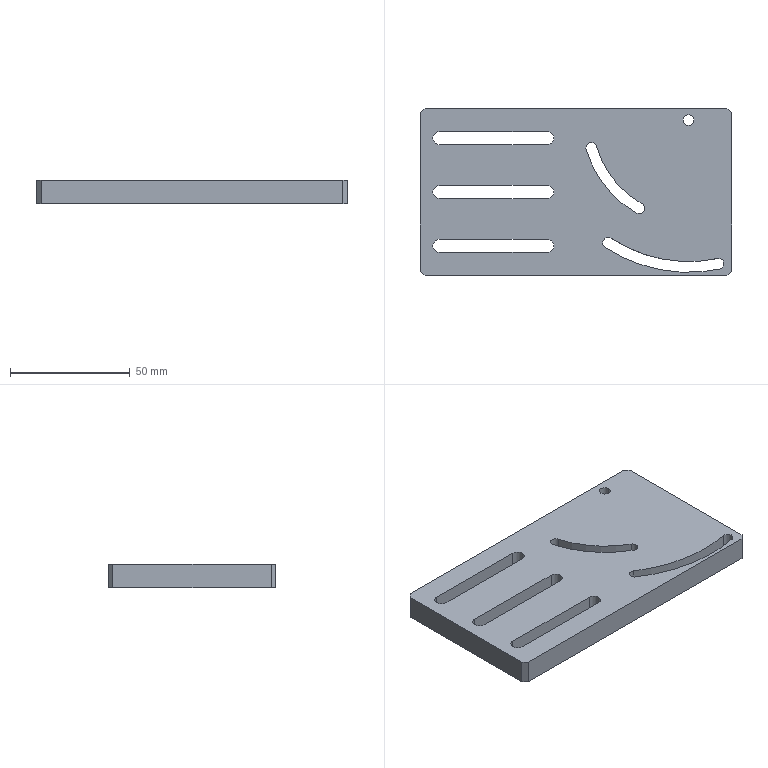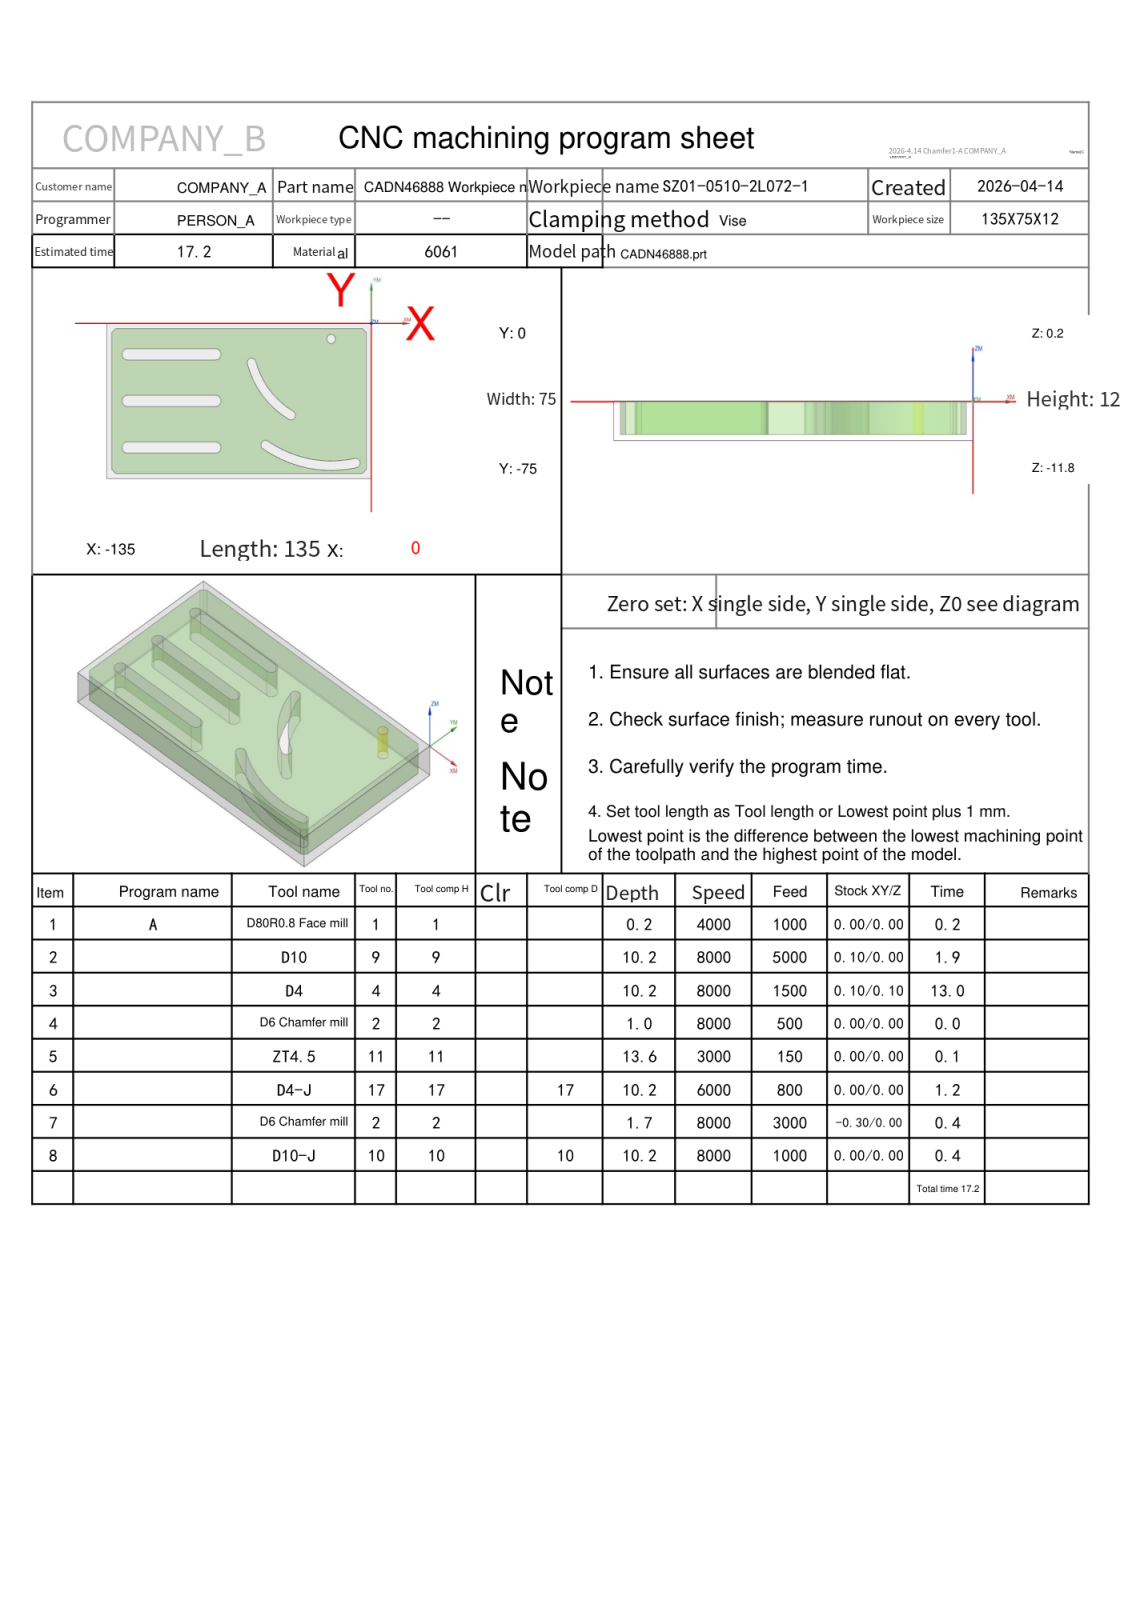NC program | NX | posted by the shop | part box 130 x 70 x 10 mm
Lines 2099 to 2533 of 2533:
N6 T17 M06
(D4-J  D=4. R=0. H=17 ce=0.00 di=0.00)
G00 G90 G54 X-32.109 Y-67.679 M03 S6000
G43 H17 Z20.
M08
Z-4.5
G01 Z-5. F800.
G41 D17
X-32.118 Y-67.728
X-32.122 Y-67.765
G03 X-31.959 Y-67.962 I.2 J0.0
X-20.5 Y-69.038 I11.459 J60.462
X-7.949 Y-67.745 I0.0 J61.538
X-7.75 Y-67.5 I-.051 J.245
X-8. Y-67.25 I-.25 J0.0
G01 X-8.051 Y-67.255
G02 X-20.5 Y-68.538 I-12.449 J59.755
X-53.951 Y-58.556 I0.0 J61.038
G01 X-54.088 Y-58.515
G03 X-54.338 Y-58.765 I0.0 J-.25
X-54.225 Y-58.974 I.25 J0.0
X-31.959 Y-67.962 I33.725 J51.474
X-31.467 Y-68.053 I11.459 J60.462
G01 X-31.432 Y-68.056
G03 X-31.235 Y-67.892 I0.0 J.2
G01 G40 X-31.226 Y-67.842
Z-4.5
G00 Z20.
X-8.196 Y-67.541
Z-9.5
G01 Z-10.
G41 D17
X-8.178 Y-67.603
G03 X-7.986 Y-67.748 I.192 J.055
G01 X-7.931 Y-67.74
X-7.913 Y-67.734
G03 X-7.75 Y-67.5 I-.087 J.234
X-8. Y-67.25 I-.25 J0.0
G01 X-8.051 Y-67.255
G02 X-20.5 Y-68.538 I-12.449 J59.755
X-53.951 Y-58.556 I0.0 J61.038
G01 X-54.088 Y-58.515
G03 X-54.338 Y-58.765 I0.0 J-.25
X-54.225 Y-58.974 I.25 J0.0
X-20.501 Y-69.038 I33.724 J51.475
X-7.931 Y-67.74 I0.0 J61.538
G01 X-7.913 Y-67.734
G03 X-7.75 Y-67.5 I-.087 J.234
G01 X-7.81 Y-67.337
X-7.962 Y-67.267
X-8.092 Y-67.316
X-8.326 Y-67.516
G40 X-8.363 Y-67.548
Z-9.5
G00 Z20.
G00 G90 X-53.685 Y-33.589 M03 S6000
Z20.
Z-4.5
G01 Z-5. F800.
G41 D17
X-53.724 Y-33.621
X-53.8 Y-33.777
X-53.756 Y-33.902
G03 X-41.121 Y-44.619 I33.256 J26.402
G01 X-41. Y-44.65
G03 X-40.75 Y-44.4 I0.0 J.25
X-40.879 Y-44.181 I-.25 J0.0
G02 X-60.848 Y-19.028 I20.379 J36.681
G03 X-61.088 Y-18.847 I-.24 J-.069
X-61.338 Y-19.097 I0.0 J-.25
G01 X-61.328 Y-19.165
G03 X-53.756 Y-33.902 I40.828 J11.665
X-53.443 Y-34.291 I33.256 J26.402
G01 X-53.288 Y-34.365
X-53.161 Y-34.32
G40 X-53.123 Y-34.288
Z-4.5
G00 Z1.
X-53.685 Y-33.589
Z-9.5
G01 Z-10.
G41 D17
X-53.724 Y-33.621
X-53.8 Y-33.777
X-53.756 Y-33.902
G03 X-41.121 Y-44.619 I33.256 J26.402
G01 X-41. Y-44.65
G03 X-40.75 Y-44.4 I0.0 J.25
X-40.879 Y-44.181 I-.25 J0.0
G02 X-60.848 Y-19.028 I20.379 J36.681
G03 X-61.088 Y-18.847 I-.24 J-.069
X-61.338 Y-19.097 I0.0 J-.25
G01 X-61.328 Y-19.165
G03 X-53.756 Y-33.902 I40.828 J11.665
X-53.443 Y-34.291 I33.256 J26.402
G01 X-53.288 Y-34.365
X-53.161 Y-34.32
G40 X-53.123 Y-34.288
Z-9.5
G00 Z20.
G00 G90 X-101.8 Y-14.5 M03 S6000
Z20.
Z-4.5
G01 Z-5. F800.
G41 D17
Y-14.45
G03 X-102. Y-14.25 I-.2 J0.0
G01 X-124.5
G03 X-125.25 Y-15. I0.0 J-.75
X-124.5 Y-15.75 I.75 J0.0
G01 X-79.5
G03 X-78.75 Y-15. I0.0 J.75
X-79.5 Y-14.25 I-.75 J0.0
G01 X-102.
X-102.5
G03 X-102.7 Y-14.45 I0.0 J-.2
G01 G40 Y-14.5
Z-4.5
G00 Z1.
X-101.8
Z-9.5
G01 Z-10.
G41 D17
Y-14.45
G03 X-102. Y-14.25 I-.2 J0.0
G01 X-124.5
G03 X-125.25 Y-15. I0.0 J-.75
X-124.5 Y-15.75 I.75 J0.0
G01 X-79.5
G03 X-78.75 Y-15. I0.0 J.75
X-79.5 Y-14.25 I-.75 J0.0
G01 X-102.
X-102.5
G03 X-102.7 Y-14.45 I0.0 J-.2
G01 G40 Y-14.5
Z-9.5
G00 Z20.
X-101.8 Y-37.
Z-4.5
G01 Z-5.
G41 D17
Y-36.95
G03 X-102. Y-36.75 I-.2 J0.0
G01 X-124.5
G03 X-125.25 Y-37.5 I0.0 J-.75
X-124.5 Y-38.25 I.75 J0.0
G01 X-79.5
G03 X-78.75 Y-37.5 I0.0 J.75
X-79.5 Y-36.75 I-.75 J0.0
G01 X-102.
X-102.5
G03 X-102.7 Y-36.95 I0.0 J-.2
G01 G40 Y-37.
Z-4.5
G00 Z1.
X-101.8
Z-9.5
G01 Z-10.
G41 D17
Y-36.95
G03 X-102. Y-36.75 I-.2 J0.0
G01 X-124.5
G03 X-125.25 Y-37.5 I0.0 J-.75
X-124.5 Y-38.25 I.75 J0.0
G01 X-79.5
G03 X-78.75 Y-37.5 I0.0 J.75
X-79.5 Y-36.75 I-.75 J0.0
G01 X-102.
X-102.5
G03 X-102.7 Y-36.95 I0.0 J-.2
G01 G40 Y-37.
Z-9.5
G00 Z20.
X-102.2 Y-60.5
Z-4.5
G01 Z-5.
G41 D17
Y-60.55
G03 X-102. Y-60.75 I.2 J0.0
G01 X-79.5
G03 X-78.75 Y-60. I0.0 J.75
X-79.5 Y-59.25 I-.75 J0.0
G01 X-124.5
G03 X-125.25 Y-60. I0.0 J-.75
X-124.5 Y-60.75 I.75 J0.0
G01 X-102.
X-101.5
G03 X-101.3 Y-60.55 I0.0 J.2
G01 G40 Y-60.5
Z-4.5
G00 Z1.
X-102.2
Z-9.5
G01 Z-10.
G41 D17
Y-60.55
G03 X-102. Y-60.75 I.2 J0.0
G01 X-79.5
G03 X-78.75 Y-60. I0.0 J.75
X-79.5 Y-59.25 I-.75 J0.0
G01 X-124.5
G03 X-125.25 Y-60. I0.0 J-.75
X-124.5 Y-60.75 I.75 J0.0
G01 X-102.
X-101.5
G03 X-101.3 Y-60.55 I0.0 J.2
G01 G40 Y-60.5
Z-9.5
G00 Z20.
G91 G28 Z0.0
M05
M09
G91 G28 Z0.0
M01
N7 T02 M06
(D6 Chamfer mill  D=6. R=0. H=02 ce=0.00 di=0.00)
G00 G90 G54 X-67.25 Y-74.628 M03 S8000
G43 H02 Z20.
M08
Z2.099
G01 Z-1.5 F3000.
G03 X-67.17 Y-74.328 I-.52 J.3
X-67.47 Y-73.808 I-.6 J0.0
G01 X-67.5 Y-73.8
X-130.5
X-130.754 Y-73.775
X-130.997 Y-73.701
X-131.222 Y-73.581
X-131.419 Y-73.419
X-133.419 Y-71.419
X-133.581 Y-71.222
X-133.701 Y-70.997
X-133.775 Y-70.754
X-133.8 Y-70.5
Y-4.5
X-133.775 Y-4.246
X-133.701 Y-4.003
X-133.581 Y-3.778
X-133.419 Y-3.581
X-131.419 Y-1.581
X-131.222 Y-1.419
X-130.997 Y-1.299
X-130.754 Y-1.225
X-130.5 Y-1.2
X-4.5
X-4.246 Y-1.225
X-4.003 Y-1.299
X-3.778 Y-1.419
X-3.581 Y-1.581
X-1.581 Y-3.581
X-1.419 Y-3.778
X-1.299 Y-4.003
X-1.225 Y-4.246
X-1.2 Y-4.5
Y-70.5
X-1.225 Y-70.754
X-1.299 Y-70.997
X-1.419 Y-71.222
X-1.581 Y-71.419
X-3.581 Y-73.419
X-3.778 Y-73.581
X-4.003 Y-73.701
X-4.246 Y-73.775
X-4.5 Y-73.8
X-67.5
X-67.53 Y-73.808
G03 X-67.83 Y-74.328 I.3 J-.52
X-67.75 Y-74.628 I.6 J0.0
G01 Z2.099
G00 Z20.
X-101.75 Y-59.378
Z2.099
G01 Z-1.5
G03 X-101.67 Y-59.078 I-.52 J.3
X-101.97 Y-58.558 I-.6 J0.0
G01 X-102. Y-58.55
X-124.5
G03 X-125.95 Y-60. I0.0 J-1.45
X-124.5 Y-61.45 I1.45 J0.0
G01 X-79.5
G03 X-78.05 Y-60. I0.0 J1.45
X-79.5 Y-58.55 I-1.45 J0.0
G01 X-102.
X-102.03 Y-58.558
G03 X-102.33 Y-59.078 I.3 J-.52
X-102.25 Y-59.378 I.6 J0.0
G01 Z2.099
G00 Z20.
Y-38.122
Z2.099
G01 Z-1.5
G03 X-102.33 Y-38.422 I.52 J-.3
X-102.03 Y-38.942 I.6 J0.0
G01 X-102. Y-38.95
X-79.5
G03 X-78.05 Y-37.5 I0.0 J1.45
X-79.5 Y-36.05 I-1.45 J0.0
G01 X-124.5
G03 X-125.95 Y-37.5 I0.0 J-1.45
X-124.5 Y-38.95 I1.45 J0.0
G01 X-102.
X-101.97 Y-38.942
G03 X-101.67 Y-38.422 I-.3 J.52
X-101.75 Y-38.122 I-.6 J0.0
G01 Z2.099
G00 Z20.
X-102.25 Y-15.622
Z2.099
G01 Z-1.5
G03 X-102.33 Y-15.922 I.52 J-.3
X-102.03 Y-16.442 I.6 J0.0
G01 X-102. Y-16.45
X-79.5
G03 X-78.05 Y-15. I0.0 J1.45
X-79.5 Y-13.55 I-1.45 J0.0
G01 X-124.5
G03 X-125.95 Y-15. I0.0 J-1.45
X-124.5 Y-16.45 I1.45 J0.0
G01 X-102.
X-101.97 Y-16.442
G03 X-101.67 Y-15.922 I-.3 J.52
X-101.75 Y-15.622 I-.6 J0.0
G01 Z2.099
G00 Z20.
X-53.826 Y-33.617
Z2.114
G01 Z-1.5
G03 X-54.326 Y-34.209 I.1 J-.592
G01 X-54.318 Y-34.309
X-54.305 Y-34.337
G03 X-41.461 Y-45.23 I33.805 J26.837
X-41. Y-45.35 I.461 J.83
X-40.05 Y-44.4 I0.0 J.95
G01 Y-44.384
X-40.087 Y-44.139
X-40.185 Y-43.911
X-40.339 Y-43.717
X-40.539 Y-43.57
G02 X-60.174 Y-18.836 I20.039 J36.07
G03 X-61.088 Y-18.147 I-.913 J-.261
X-61.771 Y-18.436 I0.0 J-.95
G01 X-61.918 Y-18.635
X-62.009 Y-18.866
X-62.038 Y-19.112
X-62.001 Y-19.358
G03 X-54.305 Y-34.337 I41.501 J11.858
G01 X-54.28 Y-34.356
G03 X-54.049 Y-34.402 I.231 J.554
X-53.495 Y-34.034 I0.0 J.6
G01 Z2.114
G00 Z20.
X-32.196 Y-67.792
Z2.113
G01 Z-1.5
G03 X-32.334 Y-68.175 I.462 J-.383
X-32.118 Y-68.637 I.6 J0.0
G01 X-32.089 Y-68.65
G03 X-20.5 Y-69.738 I11.589 J61.15
X-7.806 Y-68.43 I0.0 J62.238
X-7.05 Y-67.5 I-.194 J.93
X-7.291 Y-66.867 I-.95 J0.0
G01 X-7.479 Y-66.705
X-7.703 Y-66.598
X-7.946 Y-66.552
X-8.194 Y-66.57
G02 X-20.5 Y-67.838 I-12.306 J59.07
X-53.567 Y-57.971 I0.0 J60.338
G03 X-54.088 Y-57.815 I-.521 J-.795
X-55.038 Y-58.757 I0.0 J-.95
G01 X-55.01 Y-58.992
X-54.925 Y-59.213
X-54.788 Y-59.407
X-54.608 Y-59.56
G03 X-32.089 Y-68.65 I34.108 J52.06
G01 X-32.058 Y-68.648
G03 X-31.646 Y-68.078 I-.188 J.57
G01 X-31.676 Y-67.89
Z2.113
G00 Z20.
G00 G90 X-20.518 Y-6.95 M03 S8000
Z20.
Z-.5
G01 Z-1. F500.
X-20.55 Y-6.
G03 X-22.05 Y-7.5 I0.0 J-1.5
X-20.5 Y-9.05 I1.55 J0.0
X-18.95 Y-7.5 I0.0 J1.55
X-20.5 Y-5.95 I-1.55 J0.0
X-22.05 Y-7.5 I0.0 J-1.55
X-20.55 Y-9. I1.5 J0.0
G01 X-20.518 Y-8.05
Z-.5
G00 Z20.
G91 G28 Z0.0
M05
M09
G91 G28 Z0.0
M01
N8 T10 M06
(D10-J  D=10. R=0. H=10 ce=0.00 di=0.00)
G00 G90 G54 X-3.487 Y-78.616 M03 S8000
G43 H10 Z20.
M08
Z-9.5
G01 Z-10. F1000.
G41 D10
X-3.503 Y-78.417
G03 X-4.5 Y-77.5 I-.997 J-.083
G01 X-130.5
G02 X-134.036 Y-76.036 I0.0 J5.
G01 X-136.036 Y-74.036
G02 X-137.5 Y-70.5 I3.536 J3.536
G01 Y-4.5
G02 X-136.036 Y-.964 I5. J0.0
G01 X-134.036 Y1.036
G02 X-130.5 Y2.5 I3.536 J-3.536
G01 X-4.5
G02 X-.964 Y1.036 I0.0 J-5.
G01 X1.036 Y-.964
G02 X2.5 Y-4.5 I-3.536 J-3.536
G01 Y-70.5
G02 X1.036 Y-74.036 I-5. J0.0
G01 X-.964 Y-76.036
G02 X-4.5 Y-77.5 I-3.536 J3.536
G01 X-5.
G03 X-6. Y-78.5 I0.0 J-1.
G01 G40 Y-78.7
Z-9.5
G00 Z20.
M05
M09
G91 G28 Z0.0
G91 G28 Y0.0
M30
%